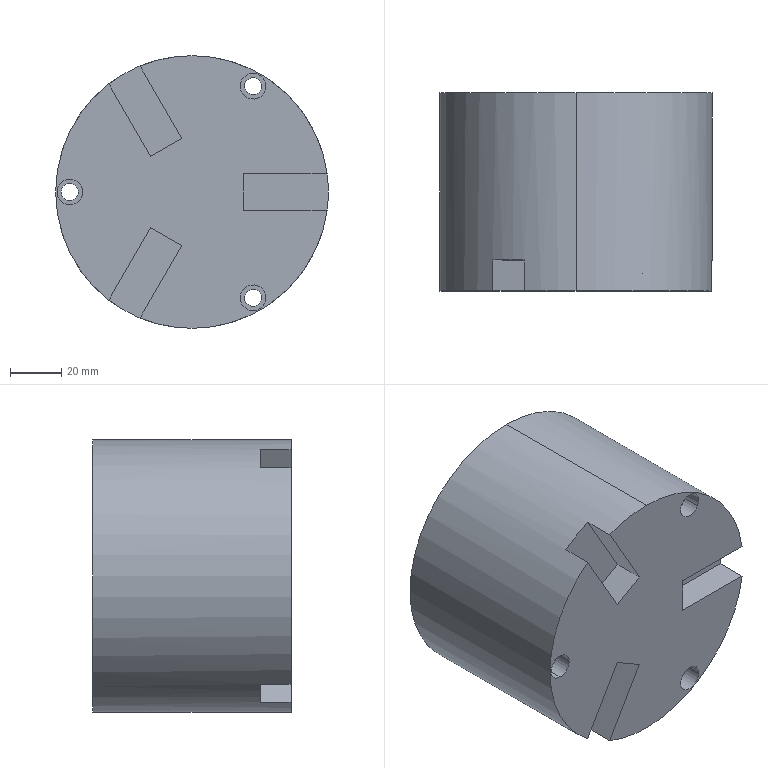Part | STEP file | PN_0062 gripper MHS3-80D | 1 solid | 31 faces | box 106 x 77 x 106 mm | volume 654143 mm3 | plane 17 | cylinder 14 | commonest cylinder face diameters 6.6 x6 10 x6 106 x2